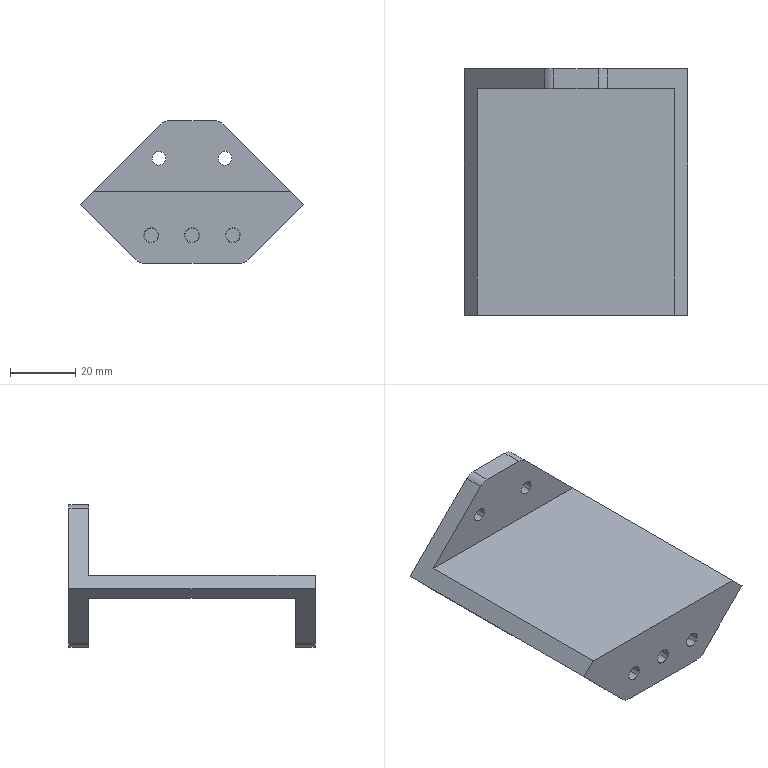NC program | NX | posted with a generic post | part box 68.307 x 75.3 x 43.668 mm
Lines 3891 to 5072 of 9000:
(ZLEVEL_PROFILE_1 , TOOL : D6R0.5)
N7750 T16 M6
N7752 G54
N7754 G17 G0 G90 X-41.212 Y19.133 B0. C0. S9500 M3
N7756 G43 Z30. H16
N7758 Z2.995
N7760 G94 G1 Z-0.005 F3500.
N7762 G3 X-38.15 Y17.111 R3.
N7764 G1 X-37.65 Y17.218
N7766 X-31.65
N7768 X-31.141 Y17.142
N7770 X-31.144 Y17.215 Z-0.008
N7772 Y17.234 Z-0.011
N7774 X-31.65 Y17.317
N7776 X-37.65
N7778 X-38.15 Y17.214
N7780 Y17.363 Z-0.02
N7782 X-38.068 Y17.383
N7784 X-37.65 Y17.419
N7786 X-31.65
N7788 X-31.202 Y17.378
N7790 X-31.151 Y17.361
N7792 X-31.144 Y17.42 Z-0.025
N7794 X-31.138 Y17.466 Z-0.03
N7796 X-31.65 Y17.518
N7798 X-37.65
N7800 X-38.081 Y17.474
N7802 X-38.151 Y17.467
N7804 X-38.195 Y17.56 Z-0.043
N7806 X-37.65 Y17.619
N7808 X-31.65
N7810 X-30.936 Y17.516
N7812 X-31.043 Y17.595 Z-0.051
N7814 X-31.151 Y17.664 Z-0.058
N7816 X-31.65 Y17.718
N7818 X-37.65
N7820 X-38.15 Y17.668
N7822 X-38.153 Y17.719 Z-0.067
N7824 X-38.156 Y17.759 Z-0.075
N7826 X-37.65 Y17.817
N7828 X-31.65
N7830 X-31.123 Y17.752
N7832 X-31.056 Y17.83 Z-0.095
N7834 X-31.65 Y17.915
N7836 X-37.65
N7838 X-38.171 Y17.85
N7840 X-38.18 Y17.908 Z-0.105
N7842 X-38.187 Y17.95 Z-0.116
N7844 X-37.65 Y18.012
N7846 X-31.65
N7848 X-30.982 Y17.916
N7850 X-30.943 Y17.96 Z-0.127
N7852 X-31.65 Y18.059
N7854 X-37.65
N7856 X-38.201 Y18.
N7858 X-38.307 Y18.027 Z-0.143
N7860 X-38.195 Y18.063
N7862 X-37.65 Y18.12
N7864 X-31.65
N7866 X-30.936 Y18.02
N7868 X-30.891 Y18.003
N7870 X-30.837 Y18.085 Z-0.168
N7872 X-30.936 Y18.116
N7874 X-31.65 Y18.215
N7876 X-37.65
N7878 X-38.354 Y18.113
N7880 X-38.269 Y18.188 Z-0.182
N7882 X-38.183 Y18.252 Z-0.196
N7884 X-37.65 Y18.311
N7886 X-31.65
N7888 X-31.109 Y18.24
N7890 Y18.338 Z-0.226
N7892 X-31.65 Y18.405
N7894 X-37.65
N7896 X-38.163 Y18.349
N7898 X-38.159 Y18.403 Z-0.242
N7900 X-38.156 Y18.45 Z-0.259
N7902 X-38.094 Y18.46
N7904 X-37.65 Y18.5
N7906 X-31.65
N7908 X-31.627 Y18.492
N7910 X-31.21 Y18.461
N7912 X-31.145 Y18.45
N7914 X-31.141 Y18.495 Z-0.275
N7916 X-31.136 Y18.539 Z-0.292
N7918 X-31.201 Y18.55
N7920 X-31.627 Y18.579
N7922 X-31.65 Y18.59
N7924 X-37.65
N7926 X-38.108 Y18.548
N7928 X-38.173 Y18.538
N7930 X-38.271 Y18.543 Z-0.302
N7932 X-38.368 Y18.538 Z-0.312
N7934 G2 X-37.65 Y18.644 R4.746
N7936 G1 X-31.65
N7938 X-30.971 Y18.557
N7940 X-30.959 Y18.595 Z-0.329
N7942 X-30.947 Y18.634 Z-0.346
N7944 X-31.65 Y18.727
N7946 X-37.65
N7948 G3 X-38.368 Y18.623 R5.11
N7950 G1 X-38.26 Y18.703 Z-0.366
N7952 X-38.151 Y18.771 Z-0.386
N7954 X-37.65 Y18.819
N7956 X-31.65
N7958 X-31.282 Y18.792
N7960 X-31.192 Y18.777
N7962 X-31.109 Y18.843 Z-0.427
N7964 X-31.65 Y18.91
N7966 X-37.65
N7968 X-38.158 Y18.855
N7970 X-38.162 Y18.905 Z-0.449
N7972 X-38.165 Y18.941 Z-0.47
N7974 X-37.65 Y18.999
N7976 X-31.65
N7978 X-31.109 Y18.93
N7980 Y18.989 Z-0.493
N7982 Y19.022 Z-0.516
N7984 X-31.65 Y19.088
N7986 X-37.65
N7988 X-38.173 Y19.031
N7990 X-38.176 Y19.077 Z-0.537
N7992 X-38.179 Y19.115 Z-0.559
N7994 X-37.65 Y19.168
N7996 X-31.65
N7998 X-31.122 Y19.115
N8000 X-31.138 Y19.2 Z-0.608
N8002 X-31.65 Y19.255
N8004 X-37.65
N8006 X-38.172 Y19.197
N8008 X-38.167 Y19.248 Z-0.633
N8010 X-38.164 Y19.282 Z-0.659
N8012 X-37.65 Y19.34
N8014 X-31.65
N8016 X-31.15 Y19.292
N8018 Y19.337 Z-0.685
N8020 X-31.151 Y19.373 Z-0.711
N8022 X-31.65 Y19.425
N8024 X-37.65
N8026 X-38.157 Y19.37
N8028 X-38.153 Y19.421 Z-0.739
N8030 X-38.15 Y19.46 Z-0.766
N8032 X-37.65 Y19.508
N8034 X-31.65
N8036 X-31.15 Y19.461
N8038 Y19.504 Z-0.794
N8040 X-31.151 Y19.535 Z-0.823
N8042 X-31.65 Y19.59
N8044 X-37.65
N8046 X-38.15 Y19.536
N8048 Y19.585 Z-0.852
N8050 Y19.615 Z-0.881
N8052 X-37.65 Y19.671
N8054 X-31.65
N8056 X-31.15 Y19.616
N8058 Y19.666 Z-0.911
N8060 Y19.699 Z-0.941
N8062 X-31.65 Y19.75
N8064 X-37.65
N8066 X-38.15 Y19.696
N8068 Y19.744 Z-0.972
N8070 Y19.78 Z-1.003
N8072 X-37.65 Y19.828
N8074 X-31.65
N8076 X-31.15 Y19.784
N8078 Y19.822 Z-1.035
N8080 Y19.86 Z-1.066
N8082 X-31.65 Y19.905
N8084 X-37.65
N8086 X-38.15 Y19.855
N8088 Y19.898 Z-1.099
N8090 Y19.928 Z-1.131
N8092 X-37.65 Y19.98
N8094 X-31.65
N8096 X-31.627 Y19.971
N8098 X-31.15 Y19.935
N8100 Y19.972 Z-1.165
N8102 Y20.011 Z-1.198
N8104 X-31.627 Y20.046
N8106 X-31.65 Y20.053
N8108 X-37.65
N8110 X-38.15 Y20.004
N8112 Y20.045 Z-1.232
N8114 Y20.081 Z-1.266
N8116 X-37.65 Y20.125
N8118 X-31.65
N8120 X-31.15 Y20.089
N8122 Y20.128 Z-1.3
N8124 Y20.166 Z-1.335
N8126 X-31.65 Y20.195
N8128 X-37.65
N8130 X-38.15 Y20.159
N8132 Y20.193 Z-1.37
N8134 Y20.231 Z-1.405
N8136 X-37.65 Y20.266
N8138 X-31.65
N8140 X-31.15 Y20.237
N8142 Y20.273 Z-1.44
N8144 Y20.308 Z-1.476
N8146 X-31.65 Y20.336
N8148 X-37.65
N8150 X-38.15 Y20.303
N8152 Y20.338 Z-1.511
N8154 Y20.375 Z-1.546
N8156 X-37.65 Y20.406
N8158 X-31.65
N8160 X-31.15 Y20.379
N8162 Y20.417 Z-1.581
N8164 Y20.45 Z-1.617
N8166 X-31.65 Y20.477
N8168 X-37.65
N8170 X-38.15 Y20.448
N8172 Y20.483 Z-1.652
N8174 Y20.52 Z-1.687
N8176 X-37.65 Y20.548
N8178 X-31.65
N8180 X-31.15 Y20.522
N8182 Y20.561 Z-1.723
N8184 Y20.594 Z-1.758
N8186 X-31.65 Y20.618
N8188 X-37.65
N8190 X-38.15 Y20.593
N8192 Y20.628 Z-1.793
N8194 Y20.665 Z-1.829
N8196 X-37.65 Y20.689
N8198 X-31.65
N8200 X-31.15 Y20.666
N8202 Y20.706 Z-1.864
N8204 Y20.738 Z-1.9
N8206 X-31.65 Y20.76
N8208 X-37.65
N8210 X-38.15 Y20.738
N8212 Y20.774 Z-1.935
N8214 Y20.81 Z-1.97
N8216 X-37.65 Y20.831
N8218 X-31.65
N8220 X-31.15 Y20.811
N8222 Y20.85 Z-2.006
N8224 Y20.883 Z-2.041
N8226 X-31.65 Y20.901
N8228 X-37.65
N8230 X-38.15 Y20.882
N8232 Y20.919 Z-2.076
N8234 Y20.955 Z-2.112
N8236 X-37.65 Y20.972
N8238 X-31.65
N8240 X-31.15 Y20.955
N8242 Y20.994 Z-2.147
N8244 Y21.027 Z-2.182
N8246 X-31.65 Y21.043
N8248 X-37.65
N8250 X-38.15 Y21.027
N8252 Y21.063 Z-2.218
N8254 Y21.099 Z-2.253
N8256 X-37.65 Y21.113
N8258 X-31.65
N8260 X-31.15 Y21.099
N8262 Y21.138 Z-2.288
N8264 Y21.171 Z-2.324
N8266 X-31.65 Y21.184
N8268 X-37.65
N8270 X-38.15 Y21.172
N8272 Y21.208 Z-2.359
N8274 Y21.244 Z-2.395
N8276 X-37.65 Y21.255
N8278 X-31.65
N8280 X-31.15 Y21.243
N8282 Y21.283 Z-2.43
N8284 Y21.315 Z-2.465
N8286 X-31.65 Y21.326
N8288 X-37.65
N8290 X-38.15 Y21.316
N8292 Y21.352 Z-2.501
N8294 Y21.388 Z-2.536
N8296 X-37.65 Y21.396
N8298 X-31.65
N8300 X-31.15 Y21.388
N8302 Y21.427 Z-2.571
N8304 Y21.46 Z-2.607
N8306 X-31.65 Y21.467
N8308 X-37.65
N8310 X-38.15 Y21.46
N8312 Y21.496 Z-2.642
N8314 Y21.532 Z-2.677
N8316 X-37.65 Y21.538
N8318 X-31.65
N8320 X-31.15 Y21.534
N8322 Y21.571 Z-2.713
N8324 Y21.603 Z-2.748
N8326 X-31.65 Y21.608
N8328 X-37.65
N8330 X-38.15 Y21.603
N8332 Y21.639 Z-2.783
N8334 Y21.674 Z-2.819
N8336 X-37.65 Y21.679
N8338 X-31.65
N8340 X-31.15 Y21.674
N8342 Y21.712 Z-2.854
N8344 Y21.745 Z-2.889
N8346 X-31.65 Y21.75
N8348 X-37.65
N8350 X-38.15 Y21.745
N8352 Y21.781 Z-2.925
N8354 Y21.817 Z-2.96
N8356 X-37.65 Y21.821
N8358 X-31.65
N8360 X-31.15 Y21.816
N8362 Y21.854 Z-2.996
N8364 Y21.886 Z-3.031
N8366 X-31.65 Y21.891
N8368 X-37.65
N8370 X-38.15 Y21.888
N8372 Y21.923 Z-3.066
N8374 Y21.958 Z-3.102
N8376 X-37.65 Y21.962
N8378 X-31.65
N8380 X-31.15 Y21.957
N8382 Y21.996 Z-3.137
N8384 Y22.028 Z-3.172
N8386 X-31.65 Y22.033
N8388 X-37.65
N8390 X-38.15 Y22.029
N8392 Y22.065 Z-3.208
N8394 Y22.1 Z-3.243
N8396 X-37.65 Y22.103
N8398 X-31.65
N8400 X-31.15 Y22.099
N8402 Y22.137 Z-3.278
N8404 Y22.17 Z-3.314
N8406 X-31.65 Y22.174
N8408 X-37.65
N8410 X-38.15 Y22.171
N8412 Y22.207 Z-3.349
N8414 Y22.242 Z-3.384
N8416 X-37.65 Y22.245
N8418 X-31.65
N8420 X-31.15 Y22.241
N8422 Y22.279 Z-3.42
N8424 Y22.311 Z-3.455
N8426 X-31.65 Y22.316
N8428 X-37.65
N8430 X-38.15 Y22.313
N8432 Y22.349 Z-3.491
N8434 Y22.384 Z-3.526
N8436 X-37.65 Y22.386
N8438 X-31.65
N8440 X-31.15 Y22.382
N8442 Y22.421 Z-3.561
N8444 Y22.453 Z-3.597
N8446 X-31.65 Y22.457
N8448 X-37.65
N8450 X-38.15 Y22.455
N8452 Y22.491 Z-3.632
N8454 Y22.526 Z-3.667
N8456 X-37.65 Y22.528
N8458 X-31.65
N8460 X-31.15 Y22.524
N8462 Y22.562 Z-3.703
N8464 Y22.595 Z-3.738
N8466 X-31.65 Y22.598
N8468 X-37.65
N8470 X-38.15 Y22.597
N8472 Y22.632 Z-3.773
N8474 Y22.668 Z-3.809
N8476 X-37.65 Y22.669
N8478 X-31.65
N8480 X-31.15 Y22.665
N8482 Y22.704 Z-3.844
N8484 Y22.736 Z-3.879
N8486 X-31.65 Y22.74
N8488 X-37.65
N8490 X-38.15 Y22.739
N8492 Y22.774 Z-3.915
N8494 Y22.809 Z-3.95
N8496 X-37.65 Y22.811
N8498 X-31.65
N8500 X-31.15 Y22.807
N8502 Y22.846 Z-3.986
N8504 Y22.878 Z-4.021
N8506 X-31.65 Y22.881
N8508 X-37.65
N8510 X-38.15 Y22.88
N8512 Y22.916 Z-4.056
N8514 Y22.951 Z-4.092
N8516 X-37.65 Y22.952
N8518 X-31.65
N8520 X-31.15 Y22.949
N8522 Y22.987 Z-4.127
N8524 Y23.019 Z-4.162
N8526 X-31.65 Y23.023
N8528 X-37.65
N8530 X-38.15 Y23.022
N8532 Y23.058 Z-4.198
N8534 Y23.093 Z-4.233
N8536 X-37.65
N8538 X-31.65
N8540 X-31.15 Y23.09
N8542 Y23.129 Z-4.268
N8544 Y23.161 Z-4.304
N8546 X-31.65 Y23.164
N8548 X-37.65
N8550 X-38.15 Y23.163
N8552 Y23.199 Z-4.339
N8554 Y23.234 Z-4.374
N8556 X-37.65 Y23.235
N8558 X-31.65
N8560 X-31.15 Y23.232
N8562 Y23.27 Z-4.41
N8564 Y23.302 Z-4.445
N8566 X-31.65 Y23.305
N8568 X-37.65
N8570 X-38.15
N8572 Y23.341 Z-4.48
N8574 Y23.376 Z-4.516
N8576 X-37.65
N8578 X-31.65
N8580 X-31.15 Y23.373
N8582 Y23.411 Z-4.551
N8584 Y23.444 Z-4.587
N8586 X-31.65 Y23.447
N8588 X-37.65
N8590 X-38.15 Y23.446
N8592 Y23.482 Z-4.622
N8594 Y23.517 Z-4.657
N8596 X-37.65 Y23.518
N8598 X-31.65
N8600 X-31.15 Y23.514
N8602 Y23.553 Z-4.693
N8604 Y23.585 Z-4.728
N8606 X-31.65 Y23.588
N8608 X-37.65
N8610 X-38.15
N8612 Y23.624 Z-4.763
N8614 Y23.659 Z-4.799
N8616 X-37.65
N8618 X-31.65
N8620 X-31.15 Y23.656
N8622 Y23.694 Z-4.834
N8624 Y23.727 Z-4.869
N8626 X-31.65 Y23.73
N8628 X-37.65
N8630 X-38.15 Y23.729
N8632 Y23.765 Z-4.905
N8634 Y23.8 Z-4.94
N8636 X-37.65
N8638 X-31.65
N8640 X-31.15 Y23.797
N8642 Y23.836 Z-4.975
N8644 Y23.868 Z-5.011
N8646 X-31.65 Y23.871
N8648 X-37.65
N8650 X-38.15
N8652 Y23.906 Z-5.046
N8654 Y23.941 Z-5.082
N8656 X-37.65 Y23.942
N8658 X-31.65
N8660 X-31.15 Y23.939
N8662 Y23.977 Z-5.117
N8664 Y24.01 Z-5.152
N8666 X-31.65 Y24.013
N8668 X-37.65
N8670 X-38.15 Y24.012
N8672 Y24.048 Z-5.188
N8674 Y24.083 Z-5.223
N8676 X-37.65
N8678 X-31.65
N8680 X-31.15 Y24.08
N8682 Y24.119 Z-5.258
N8684 Y24.151 Z-5.294
N8686 X-31.65 Y24.154
N8688 X-37.65
N8690 X-38.15
N8692 Y24.189 Z-5.329
N8694 Y24.224 Z-5.364
N8696 X-37.65 Y24.225
N8698 X-31.65
N8700 X-31.15 Y24.222
N8702 Y24.26 Z-5.4
N8704 Y24.292 Z-5.435
N8706 X-31.65 Y24.295
N8708 X-37.65
N8710 X-38.15
N8712 Y24.331 Z-5.47
N8714 Y24.366 Z-5.506
N8716 X-37.65
N8718 X-31.65
N8720 X-31.15 Y24.363
N8722 Y24.402 Z-5.541
N8724 Y24.434 Z-5.576
N8726 X-31.65 Y24.437
N8728 X-37.65
N8730 X-38.15
N8732 Y24.472 Z-5.612
N8734 Y24.507 Z-5.647
N8736 X-37.65 Y24.508
N8738 X-31.65
N8740 X-31.15 Y24.505
N8742 Y24.543 Z-5.683
N8744 Y24.575 Z-5.718
N8746 X-31.65 Y24.578
N8748 X-37.65
N8750 X-38.15
N8752 Y24.614 Z-5.753
N8754 Y24.649 Z-5.789
N8756 X-37.65
N8758 X-31.65
N8760 X-31.15 Y24.646
N8762 Y24.684 Z-5.824
N8764 Y24.717 Z-5.859
N8766 X-31.65 Y24.72
N8768 X-37.65
N8770 X-38.15 Y24.719
N8772 Y24.755 Z-5.895
N8774 Y24.79 Z-5.93
N8776 X-37.65
N8778 X-31.65
N8780 X-31.15 Y24.787
N8782 Y24.826 Z-5.965
N8784 Y24.858 Z-6.001
N8786 X-31.65 Y24.861
N8788 X-37.65
N8790 X-38.15
N8792 Y24.896 Z-6.036
N8794 Y24.932 Z-6.071
N8796 X-37.65
N8798 X-31.65
N8800 X-31.15 Y24.929
N8802 Y24.967 Z-6.107
N8804 Y25. Z-6.142
N8806 X-31.65 Y25.003
N8808 X-37.65
N8810 X-38.15 Y25.002
N8812 Y25.038 Z-6.178
N8814 Y25.073 Z-6.213
N8816 X-37.65
N8818 X-31.65
N8820 X-31.15 Y25.07
N8822 Y25.109 Z-6.248
N8824 Y25.141 Z-6.284
N8826 X-31.65 Y25.144
N8828 X-37.65
N8830 X-38.15
N8832 Y25.179 Z-6.319
N8834 Y25.214 Z-6.354
N8836 X-37.65 Y25.215
N8838 X-31.65
N8840 X-31.15 Y25.212
N8842 Y25.25 Z-6.39
N8844 Y25.282 Z-6.425
N8846 X-31.65 Y25.285
N8848 X-37.65
N8850 X-38.15
N8852 Y25.321 Z-6.46
N8854 Y25.356 Z-6.496
N8856 X-37.65
N8858 X-31.65
N8860 X-31.15 Y25.353
N8862 Y25.391 Z-6.531
N8864 Y25.424 Z-6.566
N8866 X-31.65 Y25.427
N8868 X-37.65
N8870 X-38.15
N8872 Y25.462 Z-6.602
N8874 Y25.497 Z-6.637
N8876 X-37.65 Y25.498
N8878 X-31.65
N8880 X-31.15 Y25.494
N8882 Y25.533 Z-6.673
N8884 Y25.565 Z-6.708
N8886 X-31.65 Y25.568
N8888 X-37.65
N8890 X-38.15
N8892 Y25.604 Z-6.743
N8894 Y25.639 Z-6.779
N8896 X-37.65
N8898 X-31.65
N8900 X-31.15 Y25.636
N8902 Y25.674 Z-6.814
N8904 Y25.707 Z-6.849
N8906 X-31.65 Y25.71
N8908 X-37.65
N8910 X-38.15 Y25.709
N8912 Y25.745 Z-6.885
N8914 Y25.78 Z-6.92
N8916 X-37.65
N8918 X-31.65
N8920 X-31.15 Y25.777
N8922 Y25.816 Z-6.955
N8924 Y25.848 Z-6.991
N8926 X-31.65 Y25.851
N8928 X-37.65
N8930 X-38.15
N8932 Y25.886 Z-7.026
N8934 Y25.921 Z-7.061
N8936 X-37.65 Y25.922
N8938 X-31.65
N8940 X-31.15 Y25.919
N8942 Y25.957 Z-7.097
N8944 Y25.989 Z-7.132
N8946 X-31.65 Y25.992
N8948 X-37.65
N8950 X-38.15
N8952 Y26.028 Z-7.167
N8954 Y26.063 Z-7.203
N8956 X-37.65
N8958 X-31.65
N8960 X-31.15 Y26.06
N8962 Y26.099 Z-7.238
N8964 Y26.131 Z-7.274
N8966 X-31.65 Y26.134
N8968 X-37.65
N8970 X-38.15
N8972 Y26.169 Z-7.309
N8974 Y26.204 Z-7.344
N8976 X-37.65 Y26.205
N8978 X-31.65
N8980 X-31.15 Y26.202
N8982 Y26.24 Z-7.38
N8984 Y26.272 Z-7.415
N8986 X-31.65 Y26.275
N8988 X-37.65
N8990 X-38.15
N8992 Y26.311 Z-7.45
N8994 Y26.346 Z-7.486
N8996 X-37.65
N8998 X-31.65
N9000 X-31.15 Y26.343
N9002 Y26.381 Z-7.521
N9004 Y26.414 Z-7.556
N9006 X-31.65 Y26.417
N9008 X-37.65
N9010 X-38.15 Y26.416
N9012 Y26.452 Z-7.592
N9014 Y26.487 Z-7.627
N9016 X-37.65
N9018 X-31.65
N9020 X-31.15 Y26.484
N9022 Y26.523 Z-7.662
N9024 Y26.555 Z-7.698
N9026 X-31.65 Y26.558
N9028 X-37.65
N9030 X-38.15
N9032 Y26.594 Z-7.733
N9034 Y26.629 Z-7.769
N9036 X-37.65
N9038 X-31.65
N9040 X-31.15 Y26.626
N9042 Y26.664 Z-7.804
N9044 Y26.697 Z-7.839
N9046 X-31.65 Y26.7
N9048 X-37.65
N9050 X-38.15 Y26.699
N9052 Y26.735 Z-7.875
N9054 Y26.77 Z-7.91
N9056 X-37.65
N9058 X-31.65
N9060 X-31.15 Y26.767
N9062 Y26.806 Z-7.945
N9064 Y26.838 Z-7.981
N9066 X-31.65 Y26.841
N9068 X-37.65
N9070 X-38.15
N9072 Y26.876 Z-8.016
N9074 Y26.911 Z-8.051
N9076 X-37.65 Y26.912
N9078 X-31.65
N9080 X-31.15 Y26.909
N9082 Y26.947 Z-8.087
N9084 Y26.979 Z-8.122
N9086 X-31.65 Y26.982
N9088 X-37.65
N9090 X-38.15
N9092 Y27.018 Z-8.157
N9094 Y27.053 Z-8.193
N9096 X-37.65
N9098 X-31.65
N9100 X-31.15 Y27.05
N9102 Y27.089 Z-8.228
N9104 Y27.121 Z-8.264
N9106 X-31.65 Y27.124
N9108 X-37.65
N9110 X-38.15
N9112 Y27.159 Z-8.299
N9114 Y27.194 Z-8.334
N9116 X-37.65 Y27.195
N9118 X-31.65
N9120 X-31.15 Y27.192
N9122 Y27.23 Z-8.37
N9124 Y27.262 Z-8.405
N9126 X-31.65 Y27.265
N9128 X-37.65
N9130 X-38.15
N9132 Y27.301 Z-8.44
N9134 Y27.336 Z-8.476
N9136 X-37.65
N9138 X-31.65
N9140 X-31.15 Y27.333
N9142 Y27.371 Z-8.511
N9144 Y27.404 Z-8.546
N9146 X-31.65 Y27.407
N9148 X-37.65
N9150 X-38.15 Y27.406
N9152 Y27.442 Z-8.582
N9154 Y27.477 Z-8.617
N9156 X-37.65
N9158 X-31.65
N9160 X-31.15 Y27.474
N9162 Y27.513 Z-8.652
N9164 Y27.545 Z-8.688
N9166 X-31.65 Y27.548
N9168 X-37.65
N9170 X-38.15
N9172 Y27.583 Z-8.723
N9174 Y27.619 Z-8.758
N9176 X-37.65
N9178 X-31.65
N9180 X-31.15 Y27.616
N9182 Y27.654 Z-8.794
N9184 Y27.686 Z-8.829
N9186 X-31.65 Y27.69
N9188 X-37.65
N9190 X-38.15 Y27.689
N9192 Y27.725 Z-8.865
N9194 Y27.76 Z-8.9
N9196 X-37.65
N9198 X-31.65
N9200 X-31.15 Y27.757
N9202 Y27.796 Z-8.935
N9204 Y27.828 Z-8.971
N9206 X-31.65 Y27.831
N9208 X-37.65
N9210 X-38.15
N9212 Y27.866 Z-9.006
N9214 Y27.901 Z-9.041
N9216 X-37.65 Y27.902
N9218 X-31.65
N9220 X-31.15 Y27.899
N9222 Y27.937 Z-9.077
N9224 Y27.969 Z-9.112
N9226 X-31.65 Y27.972
N9228 X-37.65
N9230 X-38.15
N9232 Y28.008 Z-9.147
N9234 Y28.043 Z-9.183
N9236 X-37.65
N9238 X-31.65
N9240 X-31.15 Y28.04
N9242 Y28.078 Z-9.218
N9244 Y28.113 Z-9.253
N9246 X-31.65 Y28.114
N9248 X-37.65
N9250 X-38.15
N9252 Y28.149 Z-9.289
N9254 Y28.184 Z-9.324
N9256 X-37.65 Y28.185
N9258 X-31.65
N9260 X-31.15 Y28.181
N9262 Y28.22 Z-9.36
N9264 Y28.252 Z-9.395
N9266 X-31.65 Y28.255
N9268 X-37.65
N9270 X-38.15
N9272 Y28.291 Z-9.43
N9274 Y28.326 Z-9.466
N9276 X-37.65
N9278 X-31.65
N9280 X-31.15 Y28.323
N9282 Y28.361 Z-9.501
N9284 Y28.394 Z-9.536
N9286 X-31.65 Y28.397
N9288 X-37.65
N9290 X-38.15 Y28.396
N9292 Y28.432 Z-9.572
N9294 Y28.467 Z-9.607
N9296 X-37.65
N9298 X-31.65
N9300 X-31.15 Y28.464
N9302 X-31.149 Y28.503 Z-9.642
N9304 Y28.535 Z-9.678
N9306 X-31.65 Y28.538
N9308 X-37.65
N9310 X-38.15
N9312 Y28.573 Z-9.713
N9314 Y28.608 Z-9.748
N9316 X-37.65 Y28.609
N9318 X-31.65
N9320 X-31.149 Y28.606
N9322 Y28.644 Z-9.784
N9324 Y28.676 Z-9.819
N9326 X-31.65 Y28.68
N9328 X-37.65
N9330 X-38.15 Y28.679
N9332 Y28.715 Z-9.854
N9334 Y28.75 Z-9.89
N9336 X-37.65
N9338 X-31.65
N9340 X-31.149 Y28.747
N9342 Y28.786 Z-9.925
N9344 Y28.818 Z-9.961
N9346 X-31.65 Y28.821
N9348 X-37.65
N9350 X-38.15
N9352 Y28.856 Z-9.996
N9354 Y28.891 Z-10.031
N9356 X-37.65 Y28.892
N9358 X-31.65
N9360 X-31.149 Y28.889
N9362 Y28.927 Z-10.067
N9364 Y28.959 Z-10.102
N9366 X-31.65 Y28.962
N9368 X-37.65
N9370 X-38.15
N9372 Y28.998 Z-10.137
N9374 Y29.033 Z-10.173
N9376 X-37.65
N9378 X-31.65
N9380 X-31.149 Y29.03
N9382 Y29.068 Z-10.208
N9384 Y29.101 Z-10.243
N9386 X-31.65 Y29.104
N9388 X-37.65
N9390 X-38.15 Y29.103
N9392 Y29.139 Z-10.279
N9394 Y29.174 Z-10.314
N9396 X-37.65
N9398 X-31.65
N9400 X-31.149 Y29.171
N9402 Y29.21 Z-10.349
N9404 Y29.242 Z-10.385
N9406 X-31.65 Y29.245
N9408 X-37.65
N9410 X-38.15
N9412 Y29.281 Z-10.42
N9414 Y29.316 Z-10.456
N9416 X-37.65
N9418 X-31.65
N9420 X-31.149 Y29.313
N9422 Y29.351 Z-10.491
N9424 Y29.384 Z-10.526
N9426 X-31.65 Y29.387
N9428 X-37.65
N9430 X-38.15 Y29.386
N9432 Y29.422 Z-10.562
N9434 Y29.457 Z-10.597
N9436 X-37.65
N9438 X-31.65
N9440 X-31.149 Y29.454
N9442 X-31.148 Y29.493 Z-10.632
N9444 Y29.525 Z-10.668
N9446 X-31.65 Y29.528
N9448 X-37.65
N9450 X-38.15
N9452 Y29.563 Z-10.703
N9454 Y29.598 Z-10.738
N9456 X-37.65 Y29.599
N9458 X-31.65
N9460 X-31.148 Y29.596
N9462 Y29.634 Z-10.774
N9464 Y29.666 Z-10.809
N9466 X-31.65 Y29.669
N9468 X-37.65
N9470 X-38.15
N9472 Y29.705 Z-10.844
N9474 Y29.74 Z-10.88
N9476 X-37.65
N9478 X-31.65
N9480 X-31.148 Y29.737
N9482 Y29.776 Z-10.915
N9484 Y29.808 Z-10.951
N9486 X-31.65 Y29.811
N9488 X-37.65
N9490 X-38.15
N9492 Y29.846 Z-10.986
N9494 Y29.881 Z-11.021
N9496 X-37.65 Y29.882
N9498 X-31.65
N9500 X-31.148 Y29.879
N9502 Y29.917 Z-11.057
N9504 Y29.949 Z-11.092
N9506 X-31.65 Y29.952
N9508 X-37.65
N9510 X-38.15
N9512 Y29.988 Z-11.127
N9514 Y30.023 Z-11.163
N9516 X-37.65
N9518 X-31.65
N9520 X-31.148 Y30.02
N9522 Y30.058 Z-11.198
N9524 Y30.091 Z-11.233
N9526 X-31.65 Y30.094
N9528 X-37.65
N9530 X-38.15 Y30.093
N9532 Y30.129 Z-11.269
N9534 Y30.164 Z-11.304
N9536 X-37.65
N9538 X-31.65
N9540 X-31.148 Y30.161
N9542 X-31.147 Y30.2 Z-11.339
N9544 Y30.232 Z-11.375
N9546 X-31.65 Y30.235
N9548 X-37.65
N9550 X-38.15
N9552 Y30.27 Z-11.41
N9554 Y30.306 Z-11.445
N9556 X-37.65
N9558 X-31.65
N9560 X-31.147 Y30.303
N9562 Y30.341 Z-11.481
N9564 Y30.374 Z-11.516
N9566 X-31.65 Y30.377
N9568 X-37.65
N9570 X-38.149 Y30.376
N9572 Y30.412 Z-11.552
N9574 Y30.447 Z-11.587
N9576 X-37.65
N9578 X-31.65
N9580 X-31.147 Y30.444
N9582 Y30.483 Z-11.622
N9584 Y30.515 Z-11.658
N9586 X-31.65 Y30.518
N9588 X-37.65
N9590 X-38.149
N9592 Y30.553 Z-11.693
N9594 Y30.588 Z-11.728
N9596 X-37.65 Y30.589
N9598 X-31.65
N9600 X-31.147 Y30.586
N9602 Y30.624 Z-11.764
N9604 X-31.146 Y30.656 Z-11.799
N9606 X-31.65 Y30.659
N9608 X-37.65
N9610 X-38.149
N9612 Y30.695 Z-11.834
N9614 Y30.73 Z-11.87
N9616 X-37.65
N9618 X-31.65
N9620 X-31.146 Y30.727
N9622 Y30.765 Z-11.905
N9624 Y30.798 Z-11.94
N9626 X-31.65 Y30.801
N9628 X-37.65
N9630 X-38.149
N9632 Y30.836 Z-11.976
N9634 Y30.871 Z-12.011
N9636 X-37.65 Y30.872
N9638 X-31.65
N9640 X-31.146 Y30.868
N9642 Y30.907 Z-12.047
N9644 Y30.939 Z-12.082
N9646 X-31.65 Y30.942
N9648 X-37.65
N9650 X-38.149
N9652 Y30.978 Z-12.117
N9654 Y31.013 Z-12.153
N9656 X-37.65
N9658 X-31.65
N9660 X-31.146 Y31.01
N9662 Y31.048 Z-12.188
N9664 Y31.081 Z-12.223
N9666 X-31.65 Y31.084
N9668 X-37.65
N9670 X-38.149 Y31.083
N9672 Y31.119 Z-12.259
N9674 Y31.154 Z-12.294
N9676 X-37.65
N9678 X-31.65
N9680 X-31.146 Y31.151
N9682 X-31.145 Y31.19 Z-12.329
N9684 Y31.222 Z-12.365
N9686 X-31.65 Y31.225
N9688 X-37.65
N9690 X-38.149
N9692 Y31.26 Z-12.4
N9694 Y31.295 Z-12.435
N9696 X-37.65 Y31.296
N9698 X-31.65
N9700 X-31.145 Y31.293
N9702 Y31.331 Z-12.471
N9704 Y31.363 Z-12.506
N9706 X-31.65 Y31.367
N9708 X-37.65
N9710 X-38.149 Y31.366
N9712 Y31.402 Z-12.541
N9714 Y31.437 Z-12.577
N9716 X-37.65
N9718 X-31.65
N9720 X-31.145 Y31.434
N9722 X-31.144 Y31.473 Z-12.612
N9724 Y31.505 Z-12.648
N9726 X-31.65 Y31.508
N9728 X-37.65
N9730 X-38.149
N9732 Y31.543 Z-12.683
N9734 Y31.578 Z-12.718
N9736 X-37.65 Y31.579
N9738 X-31.65
N9740 X-31.144 Y31.576
N9742 Y31.614 Z-12.754
N9744 Y31.646 Z-12.789
N9746 X-31.65 Y31.649
N9748 X-37.65
N9750 X-38.149
N9752 Y31.685 Z-12.824
N9754 Y31.72 Z-12.86
N9756 X-37.65
N9758 X-31.65
N9760 X-31.144 Y31.717
N9762 Y31.755 Z-12.895
N9764 X-31.143 Y31.788 Z-12.93
N9766 X-31.65 Y31.791
N9768 X-37.65
N9770 X-38.148 Y31.79
N9772 Y31.826 Z-12.966
N9774 Y31.861 Z-13.001
N9776 X-37.65
N9778 X-31.65
N9780 X-31.143 Y31.858
N9782 Y31.897 Z-13.036
N9784 Y31.929 Z-13.072
N9786 X-31.65 Y31.932
N9788 X-37.65
N9790 X-38.148
N9792 Y31.968 Z-13.107
N9794 Y32.003 Z-13.143
N9796 X-37.65
N9798 X-31.65
N9800 X-31.143 Y32.
N9802 Y32.038 Z-13.178
N9804 Y32.071 Z-13.213
N9806 X-31.65 Y32.074
N9808 X-37.65
N9810 X-38.148 Y32.073
N9812 Y32.109 Z-13.249
N9814 Y32.144 Z-13.284
N9816 X-37.65
N9818 X-31.65
N9820 X-31.142 Y32.141
N9822 Y32.18 Z-13.319
N9824 Y32.212 Z-13.355
N9826 X-31.65 Y32.215
N9828 X-37.65
N9830 X-38.148
N9832 Y32.25 Z-13.39
N9834 Y32.285 Z-13.425
N9836 X-37.65 Y32.286
N9838 X-31.65
N9840 X-31.142 Y32.283
N9842 Y32.321 Z-13.461
N9844 Y32.353 Z-13.496
N9846 X-31.65 Y32.356
N9848 X-37.65
N9850 X-38.148
N9852 Y32.392 Z-13.531
N9854 Y32.427 Z-13.567
N9856 X-37.65
N9858 X-31.65
N9860 X-31.141 Y32.424
N9862 Y32.462 Z-13.602
N9864 Y32.495 Z-13.638
N9866 X-31.65 Y32.498
N9868 X-37.65
N9870 X-38.148
N9872 Y32.533 Z-13.673
N9874 Y32.568 Z-13.708
N9876 X-37.65 Y32.569
N9878 X-31.65
N9880 X-31.141 Y32.566
N9882 Y32.604 Z-13.744
N9884 X-31.14 Y32.636 Z-13.779
N9886 X-31.65 Y32.639
N9888 X-37.65
N9890 X-38.147
N9892 Y32.675 Z-13.814
N9894 Y32.71 Z-13.85
N9896 X-37.65
N9898 X-31.65
N9900 X-31.139 Y32.707
N9902 X-31.138 Y32.745 Z-13.885
N9904 Y32.778 Z-13.92
N9906 X-31.65 Y32.781
N9908 X-37.65
N9910 X-38.147 Y32.78
N9912 Y32.816 Z-13.956
N9914 Y32.851 Z-13.991
N9916 X-37.65
N9918 X-31.65
N9920 X-31.137 Y32.848
N9922 X-31.136 Y32.887 Z-14.026
N9924 Y32.919 Z-14.062
N9926 X-31.65 Y32.922
N9928 X-37.65
N9930 X-38.147
N9932 Y32.957 Z-14.097
N9934 X-38.146 Y32.993 Z-14.132
N9936 X-37.65
N9938 X-31.65
N9940 X-31.134 Y32.99
N9942 Y33.028 Z-14.168
N9944 X-31.133 Y33.061 Z-14.203
N9946 X-31.65 Y33.064
N9948 X-37.65
N9950 X-38.146 Y33.063
N9952 Y33.099 Z-14.239
N9954 Y33.134 Z-14.274
N9956 X-37.65
N9958 X-31.65
N9960 X-31.132 Y33.131
N9962 X-31.131 Y33.17 Z-14.309
N9964 Y33.202 Z-14.345
N9966 X-31.65 Y33.205
N9968 X-37.65
N9970 X-38.146
N9972 Y33.24 Z-14.38
N9974 Y33.275 Z-14.415
N9976 X-37.65 Y33.276
N9978 X-31.65
N9980 X-31.13 Y33.273
N9982 X-31.106 Y33.343 Z-14.486
N9984 X-31.65 Y33.346
N9986 X-37.65
N9988 X-38.145
N9990 Y33.382 Z-14.521
N9992 Y33.417 Z-14.557
N9994 X-37.65
N9996 X-31.65
N9998 X-31.064 Y33.414
N10000 X-31.023 Y33.485 Z-14.627
N10002 X-31.65 Y33.488
N10004 X-37.65
N10006 X-38.145 Y33.487
N10008 Y33.523 Z-14.663
N10010 Y33.558 Z-14.698
N10012 X-37.65 Y33.559
N10014 X-31.65
N10016 X-30.982 Y33.557
N10018 X-30.941 Y33.629 Z-14.769
N10020 X-31.65
N10022 X-37.65
N10024 X-38.145
N10026 G2 X-41.047 Y35.862 R3.
N10028 G1 Z-11.769
N10030 G0 Z30.
N10032 X27.916 Y18.994
N10034 Z2.995
N10036 G1 Z-0.005
N10038 G3 X31.141 Y17.142 R3.
N10040 G1 X31.65 Y17.218
N10042 X37.65
N10044 X38.15 Y17.111
N10046 Y17.22 Z-0.008
N10048 Y17.214 Z-0.011
N10050 X37.65 Y17.317
N10052 X31.65
N10054 X31.144 Y17.234
N10056 X31.151 Y17.361 Z-0.02
N10058 X31.202 Y17.378
N10060 X31.65 Y17.419
N10062 X37.65
N10064 X38.069 Y17.383
N10066 X38.15 Y17.363
N10068 Y17.421 Z-0.025
N10070 X38.151 Y17.46 Z-0.03
N10072 X38.125 Y17.469
N10074 X37.65 Y17.518
N10076 X31.65
N10078 X31.147 Y17.467
N10080 X31.065 Y17.551 Z-0.043
N10082 X31.65 Y17.619
N10084 X37.65
N10086 X38.384 Y17.498
N10088 X38.268 Y17.59 Z-0.051
N10090 X38.15 Y17.668 Z-0.058
N10092 X37.65 Y17.718
N10094 X31.65
N10096 X31.151 Y17.664
N10098 X31.135 Y17.717 Z-0.067
N10100 X31.124 Y17.752 Z-0.075
N10102 X31.65 Y17.817
N10104 X37.65
N10106 X38.156 Y17.759